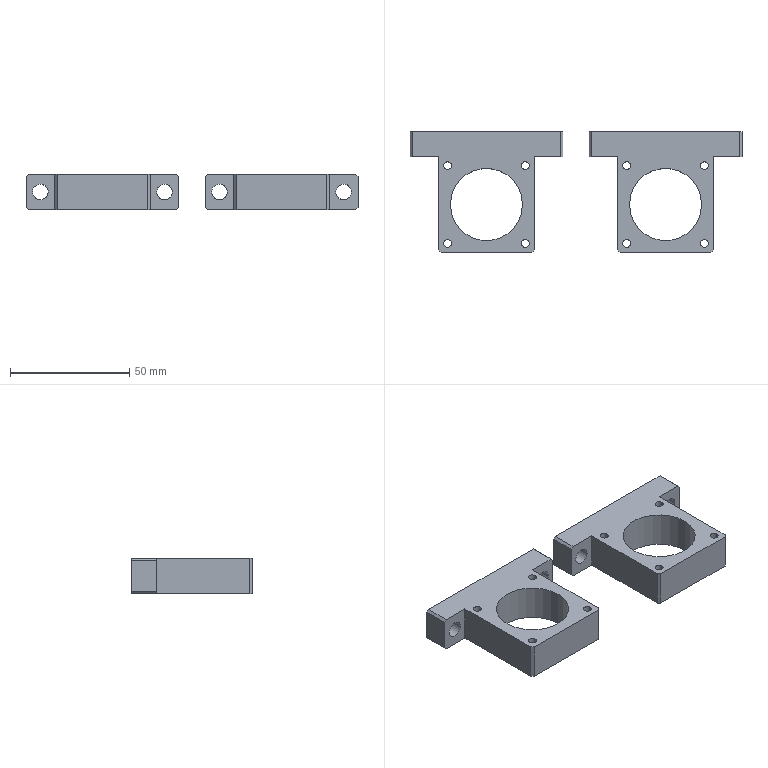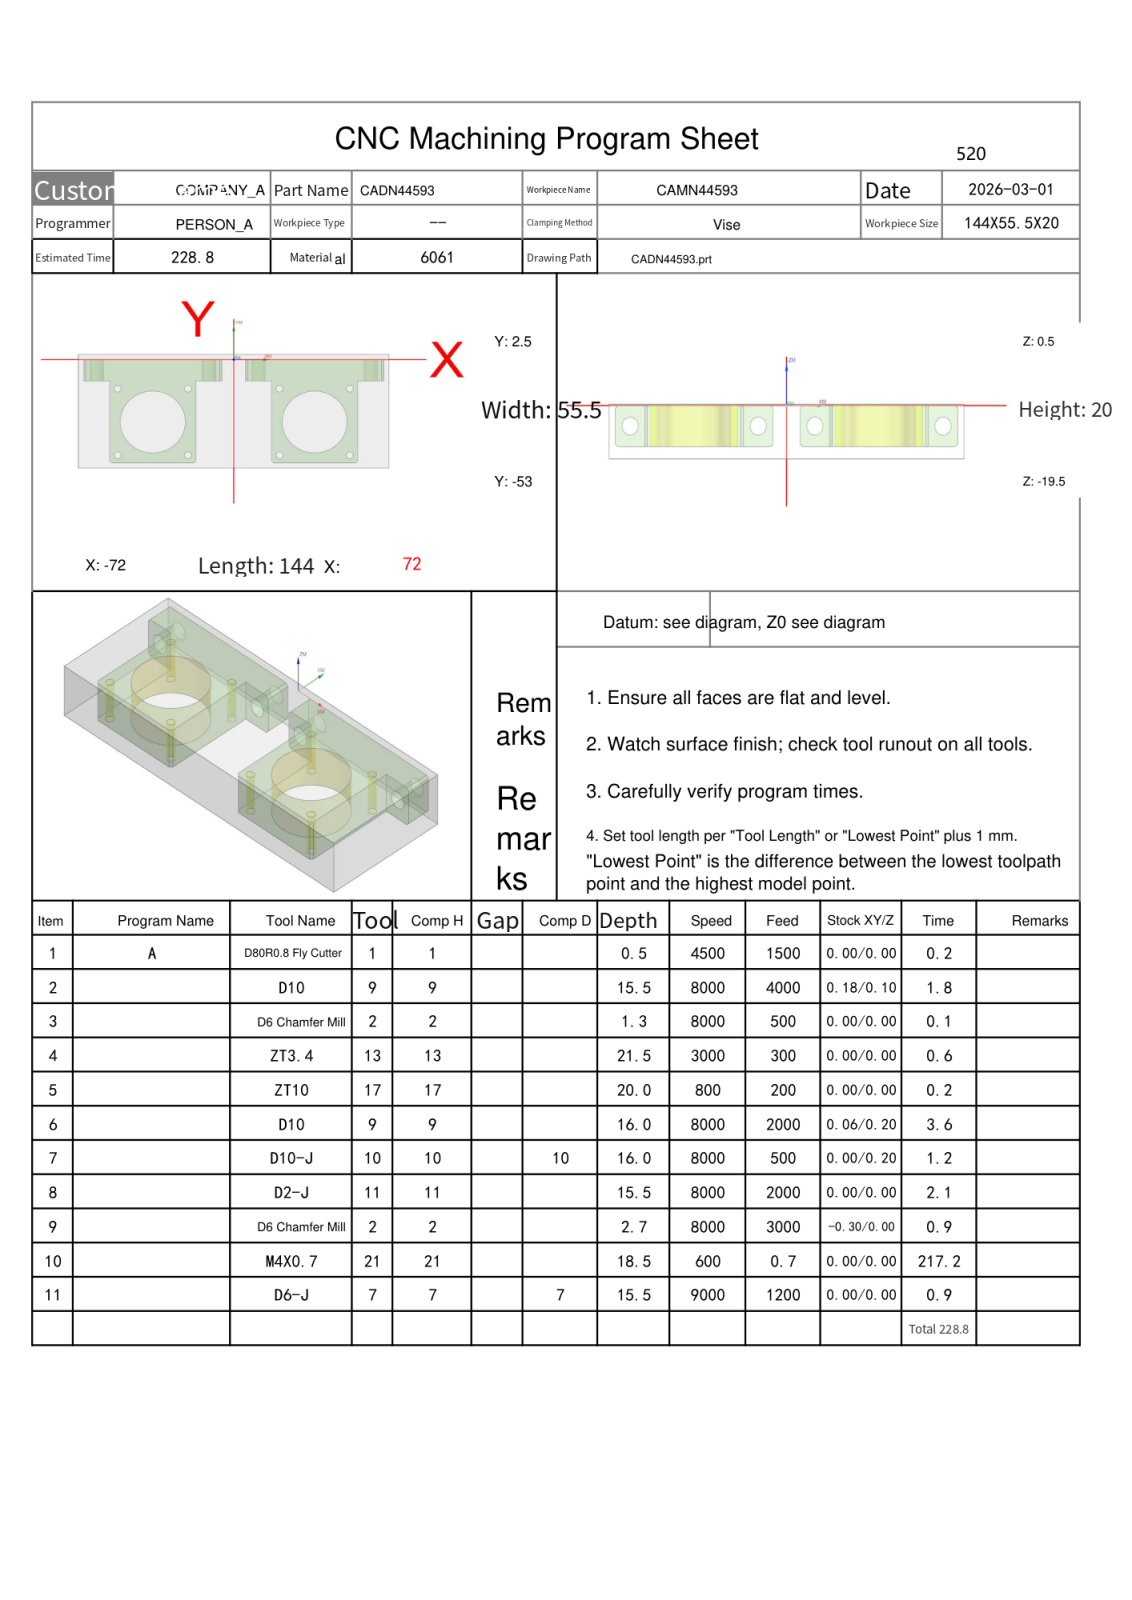NC program | NX | posted by the shop | part box 139 x 50.5 x 15 mm
Lines 1 to 35 of 10033:
%
O0001
(Machine time: 436.56 MIN)
(===Total Tool:9===)
(T1=D80R0.8 Fly Cutter D=80.  R=0.8  D-  H01 Z=0.    )
(T9=D10     D=10.  R=0.   D-  H09 Z=-15.5 )
(T2=D6 Chamfer Mill   D=6.   R=0.   D-  H02 Z=-2.2  )
(T13=ZT3.4  D=3.4  DR_a=118 D-  H13 Z=-21.  )
(T17=ZT10   D=10.  DR_a=118 D-  H17 Z=-19.5 )
(T10=D10-J  D=10.  R=0.   D10 H10 Z=-15.5 )
(T11=D2-J   D=2.   R=0.   D-  H11 Z=-15.  )
(T21=M4X0.7 D=3.3  DR_a=180 D-  H21 Z=-18.  )
(T7=D6-J    D=6.   R=0.   D7  H07 Z=-15.  )
G80 G90 G17 G49 G40
G91 G28 Z0
M01
N1 T01 M06
(D80R0.8 Fly Cutter  D=80. R=0.8 H=01 ce=0.00 di=0.00)
G00 G90 G54 X-114.5 Y-25.25 M03 S4500
G43 H01 Z50.
M08
Z2.
G01 Z0.0 F1500.
X-109.5
X109.5
X114.5
Z2.
G00 Z50.
G91 G28 Z0.0
M05
M09
G91 G28 Z0.0
M01